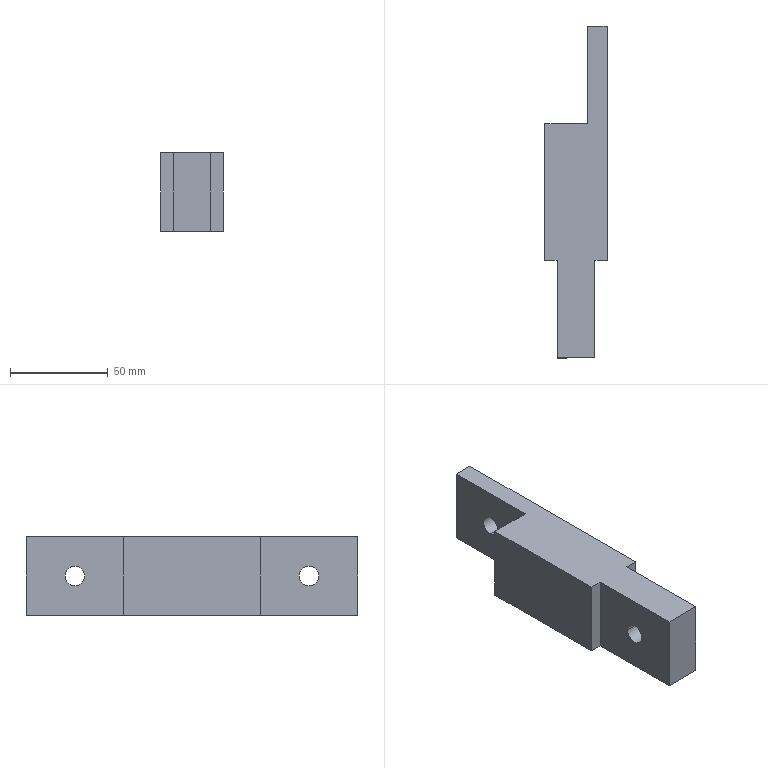Part | SolidWorks | features ICE 19, Fillet 2, MirrorPattern 1, Revolution 1, Scale 1 | 1 solid | 16 faces | box 31.854 x 170 x 40 mm | volume 145748 mm3 | plane 12 | cylinder 4 | commonest cylinder face diameters 10 x2 10.1 x2
STEP:
#1=CARTESIAN_POINT('',(-9.725,-143.23,0.));
#2=VERTEX_POINT('',#1);
#3=CARTESIAN_POINT('',(-9.725,-133.13,0.));
#4=VERTEX_POINT('',#3);
#5=CARTESIAN_POINT('',(-9.725,-138.18,0.));
#6=DIRECTION('',(1.,0.,0.));
#7=DIRECTION('',(0.,1.,0.));
#8=AXIS2_PLACEMENT_3D('',#5,#6,#7);
#9=CIRCLE('',#8,5.05);
#10=EDGE_CURVE('',#2,#4,#9,.T.);
#11=ORIENTED_EDGE('',*,*,#10,.F.);
#12=CARTESIAN_POINT('',(9.725,-143.23,0.));
#13=VERTEX_POINT('',#12);
#14=CARTESIAN_POINT('',(-15.927,-143.23,0.));
#15=DIRECTION('',(1.,0.,0.));
#16=VECTOR('',#15,1000.);
#17=LINE('',#14,#16);
#18=EDGE_CURVE('',#2,#13,#17,.T.);
#19=ORIENTED_EDGE('',*,*,#18,.T.);
#20=CARTESIAN_POINT('',(9.725,-133.13,0.));
#21=VERTEX_POINT('',#20);
#22=CARTESIAN_POINT('',(9.725,-138.18,0.));
#23=DIRECTION('',(-1.,0.,0.));
#24=DIRECTION('',(0.,-1.,0.));
#25=AXIS2_PLACEMENT_3D('',#22,#23,#24);
#26=CIRCLE('',#25,5.05);
#27=EDGE_CURVE('',#21,#13,#26,.T.);
#28=ORIENTED_EDGE('',*,*,#27,.F.);
#29=CARTESIAN_POINT('',(-15.927,-133.13,0.));
#30=DIRECTION('',(1.,0.,0.));
#31=VECTOR('',#30,1000.);
#32=LINE('',#29,#31);
#33=EDGE_CURVE('',#4,#21,#32,.T.);
#34=ORIENTED_EDGE('',*,*,#33,.F.);
#35=EDGE_LOOP('',(#11,#19,#28,#34));
#36=FACE_OUTER_BOUND('',#35,.T.);
#37=CARTESIAN_POINT('',(-15.927,-138.18,0.));
#38=DIRECTION('',(1.,0.,0.));
#39=DIRECTION('',(0.,1.,0.));
#40=AXIS2_PLACEMENT_3D('',#37,#38,#39);
#41=CYLINDRICAL_SURFACE('',#40,5.05);
#42=ADVANCED_FACE('',(#36),#41,.F.);
#43=CARTESIAN_POINT('',(5.927,-18.18,-5.));
#44=VERTEX_POINT('',#43);
#45=CARTESIAN_POINT('',(5.927,-18.18,5.));
#46=VERTEX_POINT('',#45);
#47=CARTESIAN_POINT('',(5.927,-18.18,0.));
#48=DIRECTION('',(-1.,0.,0.));
#49=DIRECTION('',(0.,0.,-1.));
#50=AXIS2_PLACEMENT_3D('',#47,#48,#49);
#51=CIRCLE('',#50,5.);
#52=EDGE_CURVE('',#44,#46,#51,.T.);
#53=ORIENTED_EDGE('',*,*,#52,.T.);
#54=CARTESIAN_POINT('',(15.927,-18.18,5.));
#55=VERTEX_POINT('',#54);
#56=CARTESIAN_POINT('',(-15.927,-18.18,5.));
#57=DIRECTION('',(1.,0.,0.));
#58=VECTOR('',#57,1000.);
#59=LINE('',#56,#58);
#60=EDGE_CURVE('',#46,#55,#59,.T.);
#61=ORIENTED_EDGE('',*,*,#60,.T.);
#62=CARTESIAN_POINT('',(15.927,-18.18,-5.));
#63=VERTEX_POINT('',#62);
#64=CARTESIAN_POINT('',(15.927,-18.18,0.));
#65=DIRECTION('',(-1.,0.,0.));
#66=DIRECTION('',(0.,0.,1.));
#67=AXIS2_PLACEMENT_3D('',#64,#65,#66);
#68=CIRCLE('',#67,5.);
#69=EDGE_CURVE('',#63,#55,#68,.T.);
#70=ORIENTED_EDGE('',*,*,#69,.F.);
#71=CARTESIAN_POINT('',(-15.927,-18.18,-5.));
#72=DIRECTION('',(1.,0.,0.));
#73=VECTOR('',#72,1000.);
#74=LINE('',#71,#73);
#75=EDGE_CURVE('',#44,#63,#74,.T.);
#76=ORIENTED_EDGE('',*,*,#75,.F.);
#77=EDGE_LOOP('',(#53,#61,#70,#76));
#78=FACE_OUTER_BOUND('',#77,.T.);
#79=CARTESIAN_POINT('',(-15.927,-18.18,0.));
#80=DIRECTION('',(1.,0.,0.));
#81=DIRECTION('',(0.,0.,-1.));
#82=AXIS2_PLACEMENT_3D('',#79,#80,#81);
#83=CYLINDRICAL_SURFACE('',#82,5.);
#84=ADVANCED_FACE('',(#78),#83,.F.);
#85=CARTESIAN_POINT('',(5.927,-43.18,-20.));
#86=VERTEX_POINT('',#85);
#87=CARTESIAN_POINT('',(5.927,-43.18,20.));
#88=VERTEX_POINT('',#87);
#89=CARTESIAN_POINT('',(5.927,-43.18,-42.771));
#90=DIRECTION('',(0.,0.,1.));
#91=VECTOR('',#90,1000.);
#92=LINE('',#89,#91);
#93=EDGE_CURVE('',#86,#88,#92,.T.);
#94=ORIENTED_EDGE('',*,*,#93,.F.);
#95=CARTESIAN_POINT('',(-15.927,-43.18,-20.));
#96=VERTEX_POINT('',#95);
#97=CARTESIAN_POINT('',(-43.18,-43.18,-20.));
#98=DIRECTION('',(-1.,0.,0.));
#99=VECTOR('',#98,1000.);
#100=LINE('',#97,#99);
#101=EDGE_CURVE('',#86,#96,#100,.T.);
#102=ORIENTED_EDGE('',*,*,#101,.T.);
#103=CARTESIAN_POINT('',(-15.927,-43.18,20.));
#104=VERTEX_POINT('',#103);
#105=CARTESIAN_POINT('',(-15.927,-43.18,-17.));
#106=DIRECTION('',(0.,0.,1.));
#107=VECTOR('',#106,1000.);
#108=LINE('',#105,#107);
#109=EDGE_CURVE('',#96,#104,#108,.T.);
#110=ORIENTED_EDGE('',*,*,#109,.T.);
#111=CARTESIAN_POINT('',(-43.18,-43.18,20.));
#112=DIRECTION('',(1.,0.,0.));
#113=VECTOR('',#112,1000.);
#114=LINE('',#111,#113);
#115=EDGE_CURVE('',#104,#88,#114,.T.);
#116=ORIENTED_EDGE('',*,*,#115,.T.);
#117=EDGE_LOOP('',(#94,#102,#110,#116));
#118=FACE_OUTER_BOUND('',#117,.T.);
#119=CARTESIAN_POINT('',(-43.18,-43.18,-17.));
#120=DIRECTION('',(0.,-1.,0.));
#121=DIRECTION('',(0.,0.,-1.));
#122=AXIS2_PLACEMENT_3D('',#119,#120,#121);
#123=PLANE('',#122);
#124=ADVANCED_FACE('',(#118),#123,.F.);
#125=ORIENTED_EDGE('',*,*,#69,.T.);
#126=CARTESIAN_POINT('',(15.927,-18.18,0.));
#127=DIRECTION('',(-1.,0.,0.));
#128=DIRECTION('',(0.,0.,1.));
#129=AXIS2_PLACEMENT_3D('',#126,#127,#128);
#130=CIRCLE('',#129,5.);
#131=EDGE_CURVE('',#55,#63,#130,.T.);
#132=ORIENTED_EDGE('',*,*,#131,.T.);
#133=EDGE_LOOP('',(#125,#132));
#134=FACE_BOUND('',#133,.T.);
#135=CARTESIAN_POINT('',(15.927,6.82,20.));
#136=VERTEX_POINT('',#135);
#137=CARTESIAN_POINT('',(15.927,-113.18,20.));
#138=VERTEX_POINT('',#137);
#139=CARTESIAN_POINT('',(15.927,20.089,20.));
#140=DIRECTION('',(0.,-1.,0.));
#141=VECTOR('',#140,1000.);
#142=LINE('',#139,#141);
#143=EDGE_CURVE('',#136,#138,#142,.T.);
#144=ORIENTED_EDGE('',*,*,#143,.T.);
#145=CARTESIAN_POINT('',(15.927,-113.18,-20.));
#146=VERTEX_POINT('',#145);
#147=CARTESIAN_POINT('',(15.927,-113.18,48.731));
#148=DIRECTION('',(0.,0.,-1.));
#149=VECTOR('',#148,1000.);
#150=LINE('',#147,#149);
#151=EDGE_CURVE('',#138,#146,#150,.T.);
#152=ORIENTED_EDGE('',*,*,#151,.T.);
#153=CARTESIAN_POINT('',(15.927,6.82,-20.));
#154=VERTEX_POINT('',#153);
#155=CARTESIAN_POINT('',(15.927,20.089,-20.));
#156=DIRECTION('',(0.,1.,0.));
#157=VECTOR('',#156,1000.);
#158=LINE('',#155,#157);
#159=EDGE_CURVE('',#146,#154,#158,.T.);
#160=ORIENTED_EDGE('',*,*,#159,.T.);
#161=CARTESIAN_POINT('',(15.927,6.82,40.135));
#162=DIRECTION('',(0.,0.,-1.));
#163=VECTOR('',#162,1000.);
#164=LINE('',#161,#163);
#165=EDGE_CURVE('',#136,#154,#164,.T.);
#166=ORIENTED_EDGE('',*,*,#165,.F.);
#167=EDGE_LOOP('',(#144,#152,#160,#166));
#168=FACE_OUTER_BOUND('',#167,.T.);
#169=CARTESIAN_POINT('',(15.927,-215.9,48.731));
#170=DIRECTION('',(-1.,0.,0.));
#171=DIRECTION('',(0.,0.,1.));
#172=AXIS2_PLACEMENT_3D('',#169,#170,#171);
#173=PLANE('',#172);
#174=ADVANCED_FACE('',(#134,#168),#173,.F.);
#175=CARTESIAN_POINT('',(-15.927,-113.18,-20.));
#176=VERTEX_POINT('',#175);
#177=CARTESIAN_POINT('',(-15.927,-215.9,-20.));
#178=DIRECTION('',(0.,-1.,0.));
#179=VECTOR('',#178,1000.);
#180=LINE('',#177,#179);
#181=EDGE_CURVE('',#96,#176,#180,.T.);
#182=ORIENTED_EDGE('',*,*,#181,.T.);
#183=CARTESIAN_POINT('',(-15.927,-113.18,20.));
#184=VERTEX_POINT('',#183);
#185=CARTESIAN_POINT('',(-15.927,-113.18,46.351));
#186=DIRECTION('',(0.,0.,1.));
#187=VECTOR('',#186,1000.);
#188=LINE('',#185,#187);
#189=EDGE_CURVE('',#176,#184,#188,.T.);
#190=ORIENTED_EDGE('',*,*,#189,.T.);
#191=CARTESIAN_POINT('',(-15.927,-215.9,20.));
#192=DIRECTION('',(0.,1.,0.));
#193=VECTOR('',#192,1000.);
#194=LINE('',#191,#193);
#195=EDGE_CURVE('',#184,#104,#194,.T.);
#196=ORIENTED_EDGE('',*,*,#195,.T.);
#197=ORIENTED_EDGE('',*,*,#109,.F.);
#198=EDGE_LOOP('',(#182,#190,#196,#197));
#199=FACE_OUTER_BOUND('',#198,.T.);
#200=CARTESIAN_POINT('',(-15.927,-215.9,46.351));
#201=DIRECTION('',(1.,0.,0.));
#202=DIRECTION('',(0.,0.,-1.));
#203=AXIS2_PLACEMENT_3D('',#200,#201,#202);
#204=PLANE('',#203);
#205=ADVANCED_FACE('',(#199),#204,.F.);
#206=ORIENTED_EDGE('',*,*,#52,.F.);
#207=CARTESIAN_POINT('',(5.927,-18.18,0.));
#208=DIRECTION('',(-1.,0.,0.));
#209=DIRECTION('',(0.,0.,-1.));
#210=AXIS2_PLACEMENT_3D('',#207,#208,#209);
#211=CIRCLE('',#210,5.);
#212=EDGE_CURVE('',#46,#44,#211,.T.);
#213=ORIENTED_EDGE('',*,*,#212,.F.);
#214=EDGE_LOOP('',(#206,#213));
#215=FACE_BOUND('',#214,.T.);
#216=CARTESIAN_POINT('',(5.927,6.82,-20.));
#217=VERTEX_POINT('',#216);
#218=CARTESIAN_POINT('',(5.927,6.82,20.));
#219=VERTEX_POINT('',#218);
#220=CARTESIAN_POINT('',(5.927,6.82,-42.771));
#221=DIRECTION('',(0.,0.,1.));
#222=VECTOR('',#221,1000.);
#223=LINE('',#220,#222);
#224=EDGE_CURVE('',#217,#219,#223,.T.);
#225=ORIENTED_EDGE('',*,*,#224,.F.);
#226=CARTESIAN_POINT('',(5.927,92.945,-20.));
#227=DIRECTION('',(0.,-1.,0.));
#228=VECTOR('',#227,1000.);
#229=LINE('',#226,#228);
#230=EDGE_CURVE('',#217,#86,#229,.T.);
#231=ORIENTED_EDGE('',*,*,#230,.T.);
#232=ORIENTED_EDGE('',*,*,#93,.T.);
#233=CARTESIAN_POINT('',(5.927,92.945,20.));
#234=DIRECTION('',(0.,1.,0.));
#235=VECTOR('',#234,1000.);
#236=LINE('',#233,#235);
#237=EDGE_CURVE('',#88,#219,#236,.T.);
#238=ORIENTED_EDGE('',*,*,#237,.T.);
#239=EDGE_LOOP('',(#225,#231,#232,#238));
#240=FACE_OUTER_BOUND('',#239,.T.);
#241=CARTESIAN_POINT('',(5.927,92.945,-42.771));
#242=DIRECTION('',(1.,0.,0.));
#243=DIRECTION('',(0.,0.,-1.));
#244=AXIS2_PLACEMENT_3D('',#241,#242,#243);
#245=PLANE('',#244);
#246=ADVANCED_FACE('',(#215,#240),#245,.F.);
#247=CARTESIAN_POINT('',(0.,6.82,-20.));
#248=DIRECTION('',(1.,0.,0.));
#249=VECTOR('',#248,1000.);
#250=LINE('',#247,#249);
#251=EDGE_CURVE('',#217,#154,#250,.T.);
#252=ORIENTED_EDGE('',*,*,#251,.F.);
#253=ORIENTED_EDGE('',*,*,#224,.T.);
#254=CARTESIAN_POINT('',(0.,6.82,20.));
#255=DIRECTION('',(-1.,0.,0.));
#256=VECTOR('',#255,1000.);
#257=LINE('',#254,#256);
#258=EDGE_CURVE('',#136,#219,#257,.T.);
#259=ORIENTED_EDGE('',*,*,#258,.F.);
#260=ORIENTED_EDGE('',*,*,#165,.T.);
#261=EDGE_LOOP('',(#252,#253,#259,#260));
#262=FACE_OUTER_BOUND('',#261,.T.);
#263=CARTESIAN_POINT('',(0.,6.82,0.));
#264=DIRECTION('',(0.,1.,0.));
#265=DIRECTION('',(0.,0.,1.));
#266=AXIS2_PLACEMENT_3D('',#263,#264,#265);
#267=PLANE('',#266);
#268=ADVANCED_FACE('',(#262),#267,.T.);
#269=ORIENTED_EDGE('',*,*,#60,.F.);
#270=ORIENTED_EDGE('',*,*,#212,.T.);
#271=ORIENTED_EDGE('',*,*,#75,.T.);
#272=ORIENTED_EDGE('',*,*,#131,.F.);
#273=EDGE_LOOP('',(#269,#270,#271,#272));
#274=FACE_OUTER_BOUND('',#273,.T.);
#275=CARTESIAN_POINT('',(-15.927,-18.18,0.));
#276=DIRECTION('',(1.,0.,0.));
#277=DIRECTION('',(0.,0.,-1.));
#278=AXIS2_PLACEMENT_3D('',#275,#276,#277);
#279=CYLINDRICAL_SURFACE('',#278,5.);
#280=ADVANCED_FACE('',(#274),#279,.F.);
#281=CARTESIAN_POINT('',(9.725,-163.18,20.));
#282=VERTEX_POINT('',#281);
#283=CARTESIAN_POINT('',(-9.725,-163.18,20.));
#284=VERTEX_POINT('',#283);
#285=CARTESIAN_POINT('',(15.927,-163.18,20.));
#286=DIRECTION('',(-1.,0.,0.));
#287=VECTOR('',#286,1000.);
#288=LINE('',#285,#287);
#289=EDGE_CURVE('',#282,#284,#288,.T.);
#290=ORIENTED_EDGE('',*,*,#289,.T.);
#291=CARTESIAN_POINT('',(-9.725,-163.18,-20.));
#292=VERTEX_POINT('',#291);
#293=CARTESIAN_POINT('',(-9.725,-163.18,-53.722));
#294=DIRECTION('',(0.,0.,-1.));
#295=VECTOR('',#294,1000.);
#296=LINE('',#293,#295);
#297=EDGE_CURVE('',#284,#292,#296,.T.);
#298=ORIENTED_EDGE('',*,*,#297,.T.);
#299=CARTESIAN_POINT('',(9.725,-163.18,-20.));
#300=VERTEX_POINT('',#299);
#301=CARTESIAN_POINT('',(15.927,-163.18,-20.));
#302=DIRECTION('',(1.,0.,0.));
#303=VECTOR('',#302,1000.);
#304=LINE('',#301,#303);
#305=EDGE_CURVE('',#292,#300,#304,.T.);
#306=ORIENTED_EDGE('',*,*,#305,.T.);
#307=CARTESIAN_POINT('',(9.725,-163.18,-53.722));
#308=DIRECTION('',(0.,0.,1.));
#309=VECTOR('',#308,1000.);
#310=LINE('',#307,#309);
#311=EDGE_CURVE('',#300,#282,#310,.T.);
#312=ORIENTED_EDGE('',*,*,#311,.T.);
#313=EDGE_LOOP('',(#290,#298,#306,#312));
#314=FACE_OUTER_BOUND('',#313,.T.);
#315=CARTESIAN_POINT('',(15.927,-163.18,-53.722));
#316=DIRECTION('',(0.,1.,0.));
#317=DIRECTION('',(0.,0.,1.));
#318=AXIS2_PLACEMENT_3D('',#315,#316,#317);
#319=PLANE('',#318);
#320=ADVANCED_FACE('',(#314),#319,.F.);
#321=CARTESIAN_POINT('',(-9.725,-113.18,20.));
#322=VERTEX_POINT('',#321);
#323=CARTESIAN_POINT('',(15.927,-113.18,20.));
#324=DIRECTION('',(1.,0.,0.));
#325=VECTOR('',#324,1000.);
#326=LINE('',#323,#325);
#327=EDGE_CURVE('',#184,#322,#326,.T.);
#328=ORIENTED_EDGE('',*,*,#327,.T.);
#329=CARTESIAN_POINT('',(-9.725,20.089,20.));
#330=DIRECTION('',(0.,-1.,0.));
#331=VECTOR('',#330,1000.);
#332=LINE('',#329,#331);
#333=EDGE_CURVE('',#322,#284,#332,.T.);
#334=ORIENTED_EDGE('',*,*,#333,.T.);
#335=ORIENTED_EDGE('',*,*,#289,.F.);
#336=CARTESIAN_POINT('',(9.725,-113.18,20.));
#337=VERTEX_POINT('',#336);
#338=CARTESIAN_POINT('',(9.725,20.089,20.));
#339=DIRECTION('',(0.,1.,0.));
#340=VECTOR('',#339,1000.);
#341=LINE('',#338,#340);
#342=EDGE_CURVE('',#282,#337,#341,.T.);
#343=ORIENTED_EDGE('',*,*,#342,.T.);
#344=CARTESIAN_POINT('',(15.927,-113.18,20.));
#345=DIRECTION('',(1.,0.,0.));
#346=VECTOR('',#345,1000.);
#347=LINE('',#344,#346);
#348=EDGE_CURVE('',#337,#138,#347,.T.);
#349=ORIENTED_EDGE('',*,*,#348,.T.);
#350=ORIENTED_EDGE('',*,*,#143,.F.);
#351=ORIENTED_EDGE('',*,*,#258,.T.);
#352=ORIENTED_EDGE('',*,*,#237,.F.);
#353=ORIENTED_EDGE('',*,*,#115,.F.);
#354=ORIENTED_EDGE('',*,*,#195,.F.);
#355=EDGE_LOOP('',(#328,#334,#335,#343,#349,#350,#351,#352,#353,#354));
#356=FACE_OUTER_BOUND('',#355,.T.);
#357=CARTESIAN_POINT('',(15.927,20.089,20.));
#358=DIRECTION('',(0.,0.,-1.));
#359=DIRECTION('',(0.,1.,0.));
#360=AXIS2_PLACEMENT_3D('',#357,#358,#359);
#361=PLANE('',#360);
#362=ADVANCED_FACE('',(#356),#361,.F.);
#363=ORIENTED_EDGE('',*,*,#305,.F.);
#364=CARTESIAN_POINT('',(-9.725,-113.18,-20.));
#365=VERTEX_POINT('',#364);
#366=CARTESIAN_POINT('',(-9.725,20.089,-20.));
#367=DIRECTION('',(0.,1.,0.));
#368=VECTOR('',#367,1000.);
#369=LINE('',#366,#368);
#370=EDGE_CURVE('',#292,#365,#369,.T.);
#371=ORIENTED_EDGE('',*,*,#370,.T.);
#372=CARTESIAN_POINT('',(-9.725,-113.18,-20.));
#373=DIRECTION('',(-1.,0.,0.));
#374=VECTOR('',#373,1000.);
#375=LINE('',#372,#374);
#376=EDGE_CURVE('',#365,#176,#375,.T.);
#377=ORIENTED_EDGE('',*,*,#376,.T.);
#378=ORIENTED_EDGE('',*,*,#181,.F.);
#379=ORIENTED_EDGE('',*,*,#101,.F.);
#380=ORIENTED_EDGE('',*,*,#230,.F.);
#381=ORIENTED_EDGE('',*,*,#251,.T.);
#382=ORIENTED_EDGE('',*,*,#159,.F.);
#383=CARTESIAN_POINT('',(9.725,-113.18,-20.));
#384=VERTEX_POINT('',#383);
#385=CARTESIAN_POINT('',(15.927,-113.18,-20.));
#386=DIRECTION('',(-1.,0.,0.));
#387=VECTOR('',#386,1000.);
#388=LINE('',#385,#387);
#389=EDGE_CURVE('',#146,#384,#388,.T.);
#390=ORIENTED_EDGE('',*,*,#389,.T.);
#391=CARTESIAN_POINT('',(9.725,-113.18,-20.));
#392=DIRECTION('',(0.,-1.,0.));
#393=VECTOR('',#392,1000.);
#394=LINE('',#391,#393);
#395=EDGE_CURVE('',#384,#300,#394,.T.);
#396=ORIENTED_EDGE('',*,*,#395,.T.);
#397=EDGE_LOOP('',(#363,#371,#377,#378,#379,#380,#381,#382,#390,#396));
#398=FACE_OUTER_BOUND('',#397,.T.);
#399=CARTESIAN_POINT('',(15.927,20.089,-20.));
#400=DIRECTION('',(0.,0.,1.));
#401=DIRECTION('',(0.,-1.,0.));
#402=AXIS2_PLACEMENT_3D('',#399,#400,#401);
#403=PLANE('',#402);
#404=ADVANCED_FACE('',(#398),#403,.F.);
#405=ORIENTED_EDGE('',*,*,#27,.T.);
#406=CARTESIAN_POINT('',(9.725,-138.18,0.));
#407=DIRECTION('',(-1.,0.,0.));
#408=DIRECTION('',(0.,-1.,0.));
#409=AXIS2_PLACEMENT_3D('',#406,#407,#408);
#410=CIRCLE('',#409,5.05);
#411=EDGE_CURVE('',#13,#21,#410,.T.);
#412=ORIENTED_EDGE('',*,*,#411,.T.);
#413=EDGE_LOOP('',(#405,#412));
#414=FACE_BOUND('',#413,.T.);
#415=ORIENTED_EDGE('',*,*,#395,.F.);
#416=CARTESIAN_POINT('',(9.725,-113.18,-20.));
#417=DIRECTION('',(0.,0.,1.));
#418=VECTOR('',#417,1000.);
#419=LINE('',#416,#418);
#420=EDGE_CURVE('',#384,#337,#419,.T.);
#421=ORIENTED_EDGE('',*,*,#420,.T.);
#422=ORIENTED_EDGE('',*,*,#342,.F.);
#423=ORIENTED_EDGE('',*,*,#311,.F.);
#424=EDGE_LOOP('',(#415,#421,#422,#423));
#425=FACE_OUTER_BOUND('',#424,.T.);
#426=CARTESIAN_POINT('',(9.725,-113.18,-20.));
#427=DIRECTION('',(-1.,0.,0.));
#428=DIRECTION('',(0.,-1.,0.));
#429=AXIS2_PLACEMENT_3D('',#426,#427,#428);
#430=PLANE('',#429);
#431=ADVANCED_FACE('',(#414,#425),#430,.F.);
#432=ORIENTED_EDGE('',*,*,#348,.F.);
#433=ORIENTED_EDGE('',*,*,#420,.F.);
#434=ORIENTED_EDGE('',*,*,#389,.F.);
#435=ORIENTED_EDGE('',*,*,#151,.F.);
#436=EDGE_LOOP('',(#432,#433,#434,#435));
#437=FACE_OUTER_BOUND('',#436,.T.);
#438=CARTESIAN_POINT('',(9.725,-113.18,-20.));
#439=DIRECTION('',(0.,1.,0.));
#440=DIRECTION('',(0.,0.,1.));
#441=AXIS2_PLACEMENT_3D('',#438,#439,#440);
#442=PLANE('',#441);
#443=ADVANCED_FACE('',(#437),#442,.F.);
#444=CARTESIAN_POINT('',(-9.725,-138.18,0.));
#445=DIRECTION('',(1.,0.,0.));
#446=DIRECTION('',(0.,1.,0.));
#447=AXIS2_PLACEMENT_3D('',#444,#445,#446);
#448=CIRCLE('',#447,5.05);
#449=EDGE_CURVE('',#4,#2,#448,.T.);
#450=ORIENTED_EDGE('',*,*,#449,.T.);
#451=ORIENTED_EDGE('',*,*,#10,.T.);
#452=EDGE_LOOP('',(#450,#451));
#453=FACE_BOUND('',#452,.T.);
#454=ORIENTED_EDGE('',*,*,#333,.F.);
#455=CARTESIAN_POINT('',(-9.725,-113.18,-20.));
#456=DIRECTION('',(0.,0.,1.));
#457=VECTOR('',#456,1000.);
#458=LINE('',#455,#457);
#459=EDGE_CURVE('',#365,#322,#458,.T.);
#460=ORIENTED_EDGE('',*,*,#459,.F.);
#461=ORIENTED_EDGE('',*,*,#370,.F.);
#462=ORIENTED_EDGE('',*,*,#297,.F.);
#463=EDGE_LOOP('',(#454,#460,#461,#462));
#464=FACE_OUTER_BOUND('',#463,.T.);
#465=CARTESIAN_POINT('',(-9.725,-113.18,-20.));
#466=DIRECTION('',(1.,0.,0.));
#467=DIRECTION('',(0.,1.,0.));
#468=AXIS2_PLACEMENT_3D('',#465,#466,#467);
#469=PLANE('',#468);
#470=ADVANCED_FACE('',(#453,#464),#469,.F.);
#471=ORIENTED_EDGE('',*,*,#376,.F.);
#472=ORIENTED_EDGE('',*,*,#459,.T.);
#473=ORIENTED_EDGE('',*,*,#327,.F.);
#474=ORIENTED_EDGE('',*,*,#189,.F.);
#475=EDGE_LOOP('',(#471,#472,#473,#474));
#476=FACE_OUTER_BOUND('',#475,.T.);
#477=CARTESIAN_POINT('',(-9.725,-113.18,-20.));
#478=DIRECTION('',(0.,1.,0.));
#479=DIRECTION('',(0.,0.,1.));
#480=AXIS2_PLACEMENT_3D('',#477,#478,#479);
#481=PLANE('',#480);
#482=ADVANCED_FACE('',(#476),#481,.F.);
#483=ORIENTED_EDGE('',*,*,#18,.F.);
#484=ORIENTED_EDGE('',*,*,#449,.F.);
#485=ORIENTED_EDGE('',*,*,#33,.T.);
#486=ORIENTED_EDGE('',*,*,#411,.F.);
#487=EDGE_LOOP('',(#483,#484,#485,#486));
#488=FACE_OUTER_BOUND('',#487,.T.);
#489=CARTESIAN_POINT('',(-15.927,-138.18,0.));
#490=DIRECTION('',(1.,0.,0.));
#491=DIRECTION('',(0.,1.,0.));
#492=AXIS2_PLACEMENT_3D('',#489,#490,#491);
#493=CYLINDRICAL_SURFACE('',#492,5.05);
#494=ADVANCED_FACE('',(#488),#493,.F.);
#495=CLOSED_SHELL('',(#42,#84,#124,#174,#205,#246,#268,#280,#320,#362,#404,#431,#443,#470,#482,#494));
#496=MANIFOLD_SOLID_BREP('',#495);
#497=CARTESIAN_POINT('',(0.,0.,0.));
#498=DIRECTION('',(0.,0.,1.));
#499=DIRECTION('',(1.,0.,0.));
#500=AXIS2_PLACEMENT_3D('',#497,#498,#499);
#501=(LENGTH_UNIT()NAMED_UNIT(*)SI_UNIT(.MILLI.,.METRE.));
#502=UNCERTAINTY_MEASURE_WITH_UNIT(LENGTH_MEASURE(0.00001),#501,'','');
#503=(NAMED_UNIT(*)PLANE_ANGLE_UNIT()SI_UNIT($,.RADIAN.));
#504=(NAMED_UNIT(*)SI_UNIT($,.STERADIAN.)SOLID_ANGLE_UNIT());
#505=(GEOMETRIC_REPRESENTATION_CONTEXT(3)GLOBAL_UNCERTAINTY_ASSIGNED_CONTEXT((#502))GLOBAL_UNIT_ASSIGNED_CONTEXT((#501,#503,#504))REPRESENTATION_CONTEXT('',''));
#506=ADVANCED_BREP_SHAPE_REPRESENTATION('',(#496,#500),#505);